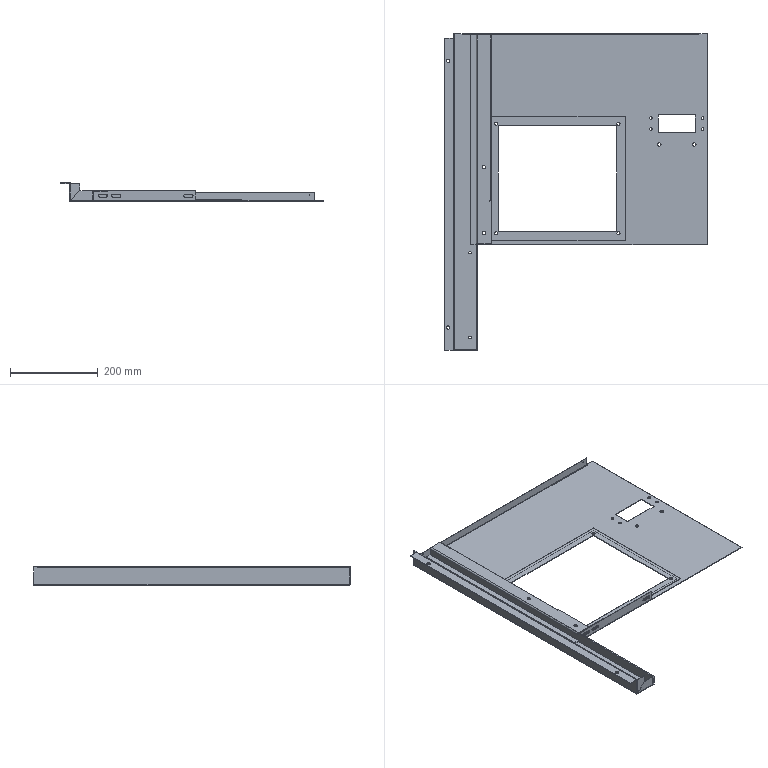Part | SolidWorks | 3 solids | 197 faces | box 600 x 723 x 41.7 mm | volume 564160 mm3 | plane 123 | cylinder 72 | spline 2 | commonest cylinder face diameters 6 x16 0.4 x9 2 x8 7.1 x8 3.4 x6 7 x6